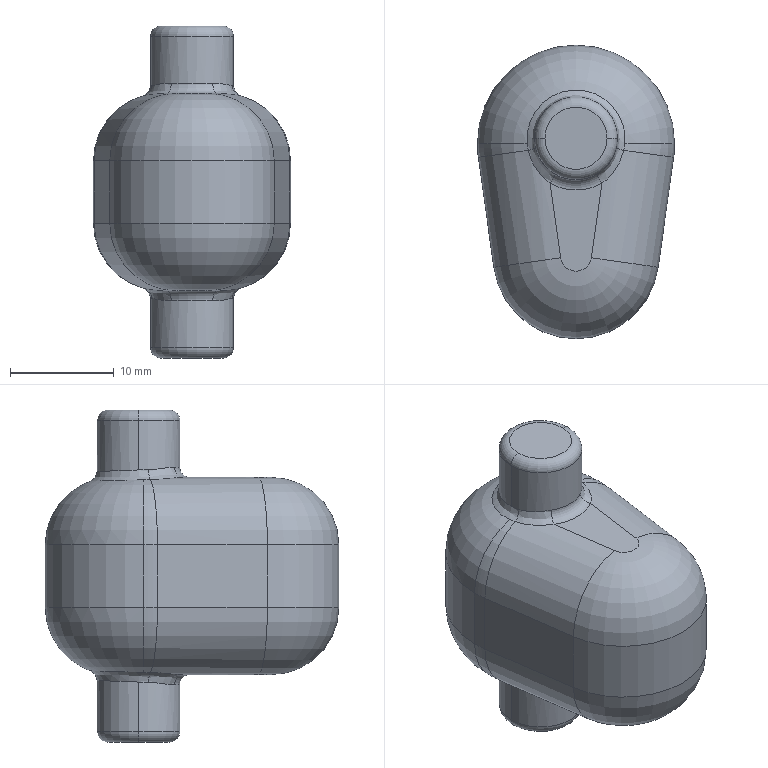Part | SolidWorks | features Fillet 3, Extrusion 1, ICE 1 | 1 solid | 38 faces | box 19 x 28.3 x 32 mm | volume 7655 mm3 | torus 14 | cylinder 12 | plane 6 | spline 6 | commonest cylinder face diameters 8 x4 13 x4 19 x3 16 x1